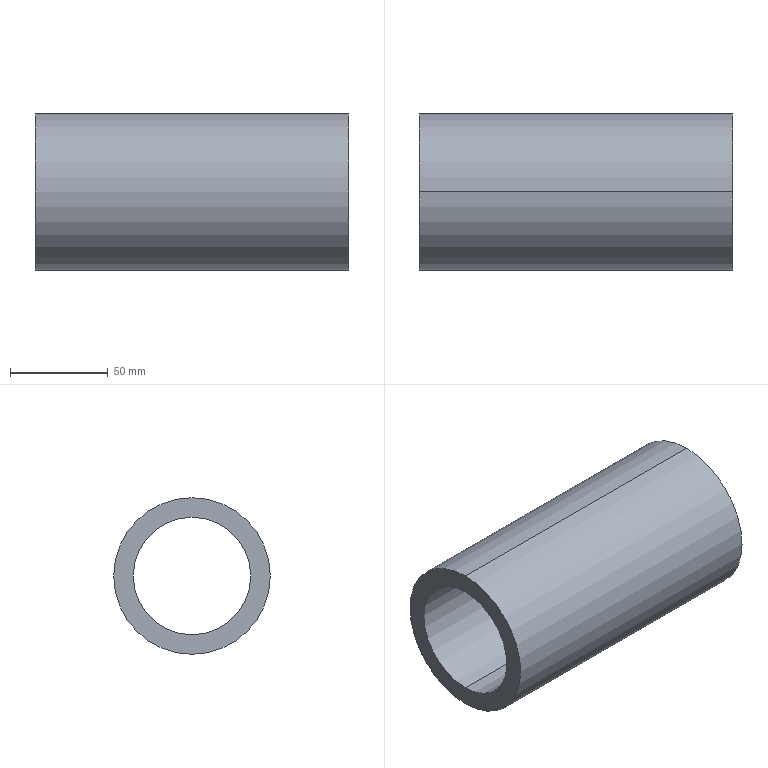Part | SolidWorks | features Extrusion 1 | 1 solid | 6 faces | box 160 x 80 x 80 mm | volume 351858 mm3 | cylinder 4 | plane 2 | commonest cylinder face diameters 60 x2 80 x2
STEP:
#1=CARTESIAN_POINT('',(160.,0.,30.));
#2=VERTEX_POINT('',#1);
#3=CARTESIAN_POINT('',(160.,0.,-30.));
#4=VERTEX_POINT('',#3);
#5=CARTESIAN_POINT('',(160.,0.,0.));
#6=DIRECTION('',(1.,0.,0.));
#7=DIRECTION('',(0.,0.,-1.));
#8=AXIS2_PLACEMENT_3D('',#5,#6,#7);
#9=CIRCLE('',#8,30.);
#10=EDGE_CURVE('',#2,#4,#9,.T.);
#11=ORIENTED_EDGE('',*,*,#10,.T.);
#12=CARTESIAN_POINT('',(0.,0.,-30.));
#13=VERTEX_POINT('',#12);
#14=CARTESIAN_POINT('',(160.,0.,-30.));
#15=DIRECTION('',(-1.,0.,0.));
#16=VECTOR('',#15,1000.);
#17=LINE('',#14,#16);
#18=EDGE_CURVE('',#4,#13,#17,.T.);
#19=ORIENTED_EDGE('',*,*,#18,.T.);
#20=CARTESIAN_POINT('',(0.,0.,30.));
#21=VERTEX_POINT('',#20);
#22=CARTESIAN_POINT('',(0.,0.,0.));
#23=DIRECTION('',(1.,0.,0.));
#24=DIRECTION('',(0.,0.,-1.));
#25=AXIS2_PLACEMENT_3D('',#22,#23,#24);
#26=CIRCLE('',#25,30.);
#27=EDGE_CURVE('',#21,#13,#26,.T.);
#28=ORIENTED_EDGE('',*,*,#27,.F.);
#29=CARTESIAN_POINT('',(160.,0.,30.));
#30=DIRECTION('',(-1.,0.,0.));
#31=VECTOR('',#30,1000.);
#32=LINE('',#29,#31);
#33=EDGE_CURVE('',#2,#21,#32,.T.);
#34=ORIENTED_EDGE('',*,*,#33,.F.);
#35=EDGE_LOOP('',(#11,#19,#28,#34));
#36=FACE_OUTER_BOUND('',#35,.T.);
#37=CARTESIAN_POINT('',(160.,0.,0.));
#38=DIRECTION('',(-1.,0.,0.));
#39=DIRECTION('',(0.,0.,1.));
#40=AXIS2_PLACEMENT_3D('',#37,#38,#39);
#41=CYLINDRICAL_SURFACE('',#40,30.);
#42=ADVANCED_FACE('',(#36),#41,.F.);
#43=CARTESIAN_POINT('',(160.,0.,-40.));
#44=VERTEX_POINT('',#43);
#45=CARTESIAN_POINT('',(160.,0.,40.));
#46=VERTEX_POINT('',#45);
#47=CARTESIAN_POINT('',(160.,0.,0.));
#48=DIRECTION('',(1.,0.,0.));
#49=DIRECTION('',(0.,0.,-1.));
#50=AXIS2_PLACEMENT_3D('',#47,#48,#49);
#51=CIRCLE('',#50,40.);
#52=EDGE_CURVE('',#44,#46,#51,.T.);
#53=ORIENTED_EDGE('',*,*,#52,.F.);
#54=CARTESIAN_POINT('',(0.,0.,-40.));
#55=VERTEX_POINT('',#54);
#56=CARTESIAN_POINT('',(160.,0.,-40.));
#57=DIRECTION('',(-1.,0.,0.));
#58=VECTOR('',#57,1000.);
#59=LINE('',#56,#58);
#60=EDGE_CURVE('',#44,#55,#59,.T.);
#61=ORIENTED_EDGE('',*,*,#60,.T.);
#62=CARTESIAN_POINT('',(0.,0.,40.));
#63=VERTEX_POINT('',#62);
#64=CARTESIAN_POINT('',(0.,0.,0.));
#65=DIRECTION('',(1.,0.,0.));
#66=DIRECTION('',(0.,0.,-1.));
#67=AXIS2_PLACEMENT_3D('',#64,#65,#66);
#68=CIRCLE('',#67,40.);
#69=EDGE_CURVE('',#55,#63,#68,.T.);
#70=ORIENTED_EDGE('',*,*,#69,.T.);
#71=CARTESIAN_POINT('',(160.,0.,40.));
#72=DIRECTION('',(-1.,0.,0.));
#73=VECTOR('',#72,1000.);
#74=LINE('',#71,#73);
#75=EDGE_CURVE('',#46,#63,#74,.T.);
#76=ORIENTED_EDGE('',*,*,#75,.F.);
#77=EDGE_LOOP('',(#53,#61,#70,#76));
#78=FACE_OUTER_BOUND('',#77,.T.);
#79=CARTESIAN_POINT('',(160.,0.,0.));
#80=DIRECTION('',(-1.,0.,0.));
#81=DIRECTION('',(0.,0.,1.));
#82=AXIS2_PLACEMENT_3D('',#79,#80,#81);
#83=CYLINDRICAL_SURFACE('',#82,40.);
#84=ADVANCED_FACE('',(#78),#83,.T.);
#85=CARTESIAN_POINT('',(160.,0.,0.));
#86=DIRECTION('',(1.,0.,0.));
#87=DIRECTION('',(0.,0.,-1.));
#88=AXIS2_PLACEMENT_3D('',#85,#86,#87);
#89=CIRCLE('',#88,40.);
#90=EDGE_CURVE('',#46,#44,#89,.T.);
#91=ORIENTED_EDGE('',*,*,#90,.T.);
#92=ORIENTED_EDGE('',*,*,#52,.T.);
#93=EDGE_LOOP('',(#91,#92));
#94=FACE_OUTER_BOUND('',#93,.T.);
#95=ORIENTED_EDGE('',*,*,#10,.F.);
#96=CARTESIAN_POINT('',(160.,0.,0.));
#97=DIRECTION('',(1.,0.,0.));
#98=DIRECTION('',(0.,0.,-1.));
#99=AXIS2_PLACEMENT_3D('',#96,#97,#98);
#100=CIRCLE('',#99,30.);
#101=EDGE_CURVE('',#4,#2,#100,.T.);
#102=ORIENTED_EDGE('',*,*,#101,.F.);
#103=EDGE_LOOP('',(#95,#102));
#104=FACE_BOUND('',#103,.T.);
#105=CARTESIAN_POINT('',(160.,0.,0.));
#106=DIRECTION('',(1.,0.,0.));
#107=DIRECTION('',(0.,0.,-1.));
#108=AXIS2_PLACEMENT_3D('',#105,#106,#107);
#109=PLANE('',#108);
#110=ADVANCED_FACE('',(#94,#104),#109,.T.);
#111=CARTESIAN_POINT('',(0.,0.,0.));
#112=DIRECTION('',(1.,0.,0.));
#113=DIRECTION('',(0.,0.,-1.));
#114=AXIS2_PLACEMENT_3D('',#111,#112,#113);
#115=CIRCLE('',#114,40.);
#116=EDGE_CURVE('',#63,#55,#115,.T.);
#117=ORIENTED_EDGE('',*,*,#116,.F.);
#118=ORIENTED_EDGE('',*,*,#69,.F.);
#119=EDGE_LOOP('',(#117,#118));
#120=FACE_OUTER_BOUND('',#119,.T.);
#121=ORIENTED_EDGE('',*,*,#27,.T.);
#122=CARTESIAN_POINT('',(0.,0.,0.));
#123=DIRECTION('',(1.,0.,0.));
#124=DIRECTION('',(0.,0.,-1.));
#125=AXIS2_PLACEMENT_3D('',#122,#123,#124);
#126=CIRCLE('',#125,30.);
#127=EDGE_CURVE('',#13,#21,#126,.T.);
#128=ORIENTED_EDGE('',*,*,#127,.T.);
#129=EDGE_LOOP('',(#121,#128));
#130=FACE_BOUND('',#129,.T.);
#131=CARTESIAN_POINT('',(0.,0.,0.));
#132=DIRECTION('',(1.,0.,0.));
#133=DIRECTION('',(0.,0.,-1.));
#134=AXIS2_PLACEMENT_3D('',#131,#132,#133);
#135=PLANE('',#134);
#136=ADVANCED_FACE('',(#120,#130),#135,.F.);
#137=ORIENTED_EDGE('',*,*,#60,.F.);
#138=ORIENTED_EDGE('',*,*,#90,.F.);
#139=ORIENTED_EDGE('',*,*,#75,.T.);
#140=ORIENTED_EDGE('',*,*,#116,.T.);
#141=EDGE_LOOP('',(#137,#138,#139,#140));
#142=FACE_OUTER_BOUND('',#141,.T.);
#143=CARTESIAN_POINT('',(160.,0.,0.));
#144=DIRECTION('',(-1.,0.,0.));
#145=DIRECTION('',(0.,0.,1.));
#146=AXIS2_PLACEMENT_3D('',#143,#144,#145);
#147=CYLINDRICAL_SURFACE('',#146,40.);
#148=ADVANCED_FACE('',(#142),#147,.T.);
#149=ORIENTED_EDGE('',*,*,#18,.F.);
#150=ORIENTED_EDGE('',*,*,#101,.T.);
#151=ORIENTED_EDGE('',*,*,#33,.T.);
#152=ORIENTED_EDGE('',*,*,#127,.F.);
#153=EDGE_LOOP('',(#149,#150,#151,#152));
#154=FACE_OUTER_BOUND('',#153,.T.);
#155=CARTESIAN_POINT('',(160.,0.,0.));
#156=DIRECTION('',(-1.,0.,0.));
#157=DIRECTION('',(0.,0.,1.));
#158=AXIS2_PLACEMENT_3D('',#155,#156,#157);
#159=CYLINDRICAL_SURFACE('',#158,30.);
#160=ADVANCED_FACE('',(#154),#159,.F.);
#161=CLOSED_SHELL('',(#42,#84,#110,#136,#148,#160));
#162=MANIFOLD_SOLID_BREP('',#161);
#163=CARTESIAN_POINT('',(0.,0.,0.));
#164=DIRECTION('',(0.,0.,1.));
#165=DIRECTION('',(1.,0.,0.));
#166=AXIS2_PLACEMENT_3D('',#163,#164,#165);
#167=(LENGTH_UNIT()NAMED_UNIT(*)SI_UNIT(.MILLI.,.METRE.));
#168=UNCERTAINTY_MEASURE_WITH_UNIT(LENGTH_MEASURE(0.00001),#167,'','');
#169=(NAMED_UNIT(*)PLANE_ANGLE_UNIT()SI_UNIT($,.RADIAN.));
#170=(NAMED_UNIT(*)SI_UNIT($,.STERADIAN.)SOLID_ANGLE_UNIT());
#171=(GEOMETRIC_REPRESENTATION_CONTEXT(3)GLOBAL_UNCERTAINTY_ASSIGNED_CONTEXT((#168))GLOBAL_UNIT_ASSIGNED_CONTEXT((#167,#169,#170))REPRESENTATION_CONTEXT('',''));
#172=ADVANCED_BREP_SHAPE_REPRESENTATION('',(#162,#166),#171);